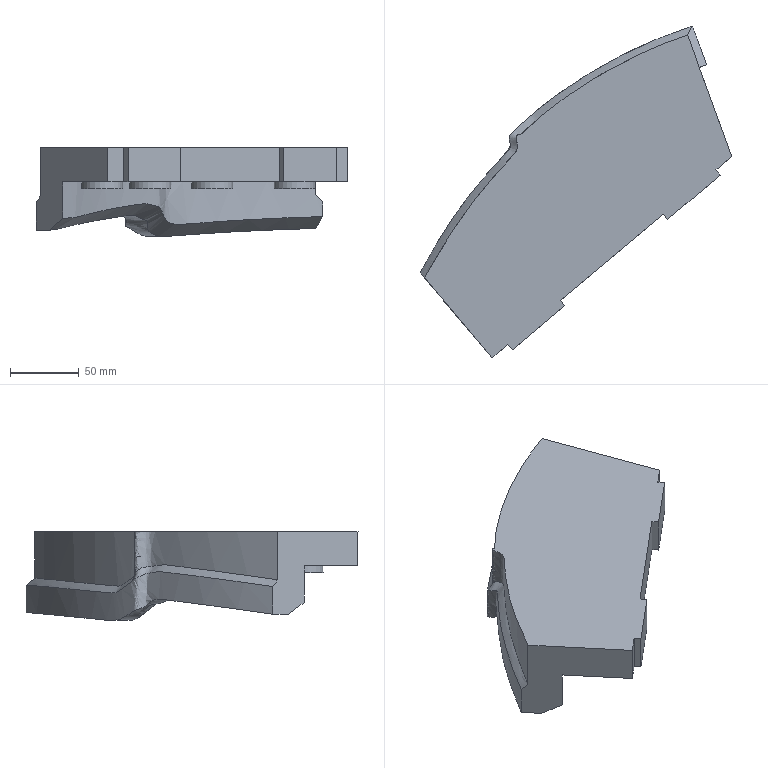Part | NX | features solid 2 | 1 solid | 32 faces | box 226.565 x 241.406 x 64.697 mm | volume 876071 mm3 | plane 20 | spline 7 | cylinder 5 | commonest cylinder face diameters 30 x5